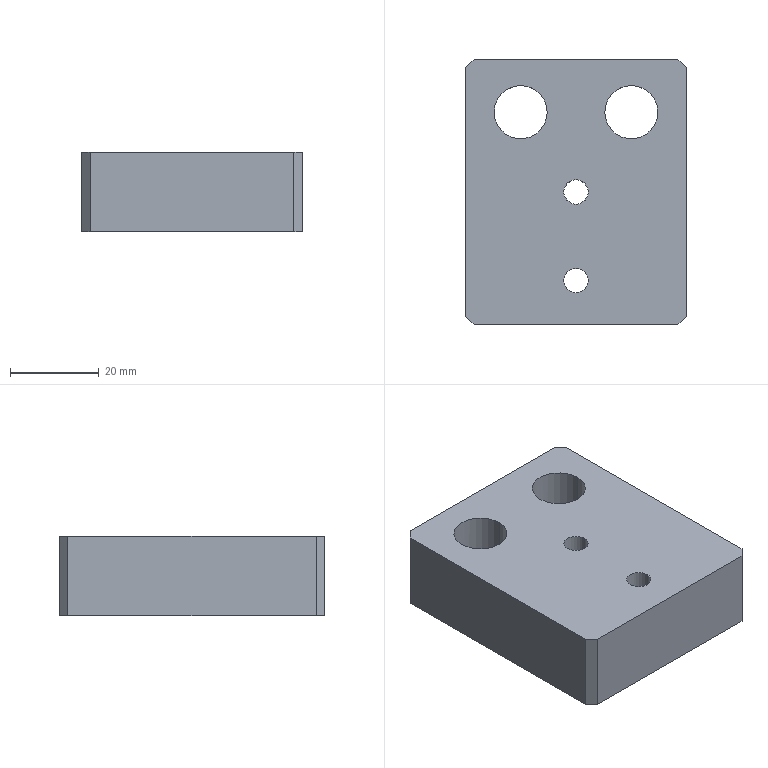Part | SolidWorks | features BaseBody 1 | 1 solid | 28 faces | box 50 x 60 x 18 mm | volume 48136 mm3 | cylinder 16 | plane 12 | commonest cylinder face diameters 4.2 x4 5.5 x4 10 x4 12 x4
STEP:
#1=CARTESIAN_POINT('',(5.,10.,-3.3));
#2=VERTEX_POINT('',#1);
#3=CARTESIAN_POINT('',(-5.,10.,-3.3));
#4=VERTEX_POINT('',#3);
#5=CARTESIAN_POINT('',(0.,10.,-3.3));
#6=DIRECTION('',(0.,0.,-1.));
#7=DIRECTION('',(-1.,0.,0.));
#8=AXIS2_PLACEMENT_3D('',#5,#6,#7);
#9=CIRCLE('',#8,5.);
#10=EDGE_CURVE('',#2,#4,#9,.T.);
#11=ORIENTED_EDGE('',*,*,#10,.F.);
#12=CARTESIAN_POINT('',(5.,10.,-9.));
#13=VERTEX_POINT('',#12);
#14=CARTESIAN_POINT('',(5.,10.,-9.));
#15=DIRECTION('',(0.,0.,-1.));
#16=VECTOR('',#15,1000.);
#17=LINE('',#14,#16);
#18=EDGE_CURVE('',#2,#13,#17,.T.);
#19=ORIENTED_EDGE('',*,*,#18,.T.);
#20=CARTESIAN_POINT('',(-5.,10.,-9.));
#21=VERTEX_POINT('',#20);
#22=CARTESIAN_POINT('',(0.,10.,-9.));
#23=DIRECTION('',(0.,0.,-1.));
#24=DIRECTION('',(-1.,0.,0.));
#25=AXIS2_PLACEMENT_3D('',#22,#23,#24);
#26=CIRCLE('',#25,5.);
#27=EDGE_CURVE('',#13,#21,#26,.T.);
#28=ORIENTED_EDGE('',*,*,#27,.T.);
#29=CARTESIAN_POINT('',(-5.,10.,-9.));
#30=DIRECTION('',(0.,0.,-1.));
#31=VECTOR('',#30,1000.);
#32=LINE('',#29,#31);
#33=EDGE_CURVE('',#4,#21,#32,.T.);
#34=ORIENTED_EDGE('',*,*,#33,.F.);
#35=EDGE_LOOP('',(#11,#19,#28,#34));
#36=FACE_OUTER_BOUND('',#35,.T.);
#37=CARTESIAN_POINT('',(0.,10.,-9.));
#38=DIRECTION('',(0.,0.,-1.));
#39=DIRECTION('',(-1.,0.,0.));
#40=AXIS2_PLACEMENT_3D('',#37,#38,#39);
#41=CYLINDRICAL_SURFACE('',#40,5.);
#42=ADVANCED_FACE('',(#36),#41,.F.);
#43=CARTESIAN_POINT('',(2.75,10.,9.));
#44=VERTEX_POINT('',#43);
#45=CARTESIAN_POINT('',(-2.75,10.,9.));
#46=VERTEX_POINT('',#45);
#47=CARTESIAN_POINT('',(0.,10.,9.));
#48=DIRECTION('',(0.,0.,-1.));
#49=DIRECTION('',(-1.,0.,0.));
#50=AXIS2_PLACEMENT_3D('',#47,#48,#49);
#51=CIRCLE('',#50,2.75);
#52=EDGE_CURVE('',#44,#46,#51,.T.);
#53=ORIENTED_EDGE('',*,*,#52,.F.);
#54=CARTESIAN_POINT('',(2.75,10.,-3.3));
#55=VERTEX_POINT('',#54);
#56=CARTESIAN_POINT('',(2.75,10.,-9.));
#57=DIRECTION('',(0.,0.,-1.));
#58=VECTOR('',#57,1000.);
#59=LINE('',#56,#58);
#60=EDGE_CURVE('',#44,#55,#59,.T.);
#61=ORIENTED_EDGE('',*,*,#60,.T.);
#62=CARTESIAN_POINT('',(-2.75,10.,-3.3));
#63=VERTEX_POINT('',#62);
#64=CARTESIAN_POINT('',(0.,10.,-3.3));
#65=DIRECTION('',(0.,0.,-1.));
#66=DIRECTION('',(-1.,0.,0.));
#67=AXIS2_PLACEMENT_3D('',#64,#65,#66);
#68=CIRCLE('',#67,2.75);
#69=EDGE_CURVE('',#55,#63,#68,.T.);
#70=ORIENTED_EDGE('',*,*,#69,.T.);
#71=CARTESIAN_POINT('',(-2.75,10.,-9.));
#72=DIRECTION('',(0.,0.,-1.));
#73=VECTOR('',#72,1000.);
#74=LINE('',#71,#73);
#75=EDGE_CURVE('',#46,#63,#74,.T.);
#76=ORIENTED_EDGE('',*,*,#75,.F.);
#77=EDGE_LOOP('',(#53,#61,#70,#76));
#78=FACE_OUTER_BOUND('',#77,.T.);
#79=CARTESIAN_POINT('',(0.,10.,-9.));
#80=DIRECTION('',(0.,0.,-1.));
#81=DIRECTION('',(-1.,0.,0.));
#82=AXIS2_PLACEMENT_3D('',#79,#80,#81);
#83=CYLINDRICAL_SURFACE('',#82,2.75);
#84=ADVANCED_FACE('',(#78),#83,.F.);
#85=CARTESIAN_POINT('',(5.,30.,-3.3));
#86=VERTEX_POINT('',#85);
#87=CARTESIAN_POINT('',(-5.,30.,-3.3));
#88=VERTEX_POINT('',#87);
#89=CARTESIAN_POINT('',(0.,30.,-3.3));
#90=DIRECTION('',(0.,0.,-1.));
#91=DIRECTION('',(-1.,0.,0.));
#92=AXIS2_PLACEMENT_3D('',#89,#90,#91);
#93=CIRCLE('',#92,5.);
#94=EDGE_CURVE('',#86,#88,#93,.T.);
#95=ORIENTED_EDGE('',*,*,#94,.F.);
#96=CARTESIAN_POINT('',(5.,30.,-9.));
#97=VERTEX_POINT('',#96);
#98=CARTESIAN_POINT('',(5.,30.,-9.));
#99=DIRECTION('',(0.,0.,-1.));
#100=VECTOR('',#99,1000.);
#101=LINE('',#98,#100);
#102=EDGE_CURVE('',#86,#97,#101,.T.);
#103=ORIENTED_EDGE('',*,*,#102,.T.);
#104=CARTESIAN_POINT('',(-5.,30.,-9.));
#105=VERTEX_POINT('',#104);
#106=CARTESIAN_POINT('',(0.,30.,-9.));
#107=DIRECTION('',(0.,0.,-1.));
#108=DIRECTION('',(-1.,0.,0.));
#109=AXIS2_PLACEMENT_3D('',#106,#107,#108);
#110=CIRCLE('',#109,5.);
#111=EDGE_CURVE('',#97,#105,#110,.T.);
#112=ORIENTED_EDGE('',*,*,#111,.T.);
#113=CARTESIAN_POINT('',(-5.,30.,-9.));
#114=DIRECTION('',(0.,0.,-1.));
#115=VECTOR('',#114,1000.);
#116=LINE('',#113,#115);
#117=EDGE_CURVE('',#88,#105,#116,.T.);
#118=ORIENTED_EDGE('',*,*,#117,.F.);
#119=EDGE_LOOP('',(#95,#103,#112,#118));
#120=FACE_OUTER_BOUND('',#119,.T.);
#121=CARTESIAN_POINT('',(0.,30.,-9.));
#122=DIRECTION('',(0.,0.,-1.));
#123=DIRECTION('',(-1.,0.,0.));
#124=AXIS2_PLACEMENT_3D('',#121,#122,#123);
#125=CYLINDRICAL_SURFACE('',#124,5.);
#126=ADVANCED_FACE('',(#120),#125,.F.);
#127=CARTESIAN_POINT('',(2.75,30.,9.));
#128=VERTEX_POINT('',#127);
#129=CARTESIAN_POINT('',(-2.75,30.,9.));
#130=VERTEX_POINT('',#129);
#131=CARTESIAN_POINT('',(0.,30.,9.));
#132=DIRECTION('',(0.,0.,-1.));
#133=DIRECTION('',(-1.,0.,0.));
#134=AXIS2_PLACEMENT_3D('',#131,#132,#133);
#135=CIRCLE('',#134,2.75);
#136=EDGE_CURVE('',#128,#130,#135,.T.);
#137=ORIENTED_EDGE('',*,*,#136,.F.);
#138=CARTESIAN_POINT('',(2.75,30.,-3.3));
#139=VERTEX_POINT('',#138);
#140=CARTESIAN_POINT('',(2.75,30.,-9.));
#141=DIRECTION('',(0.,0.,-1.));
#142=VECTOR('',#141,1000.);
#143=LINE('',#140,#142);
#144=EDGE_CURVE('',#128,#139,#143,.T.);
#145=ORIENTED_EDGE('',*,*,#144,.T.);
#146=CARTESIAN_POINT('',(-2.75,30.,-3.3));
#147=VERTEX_POINT('',#146);
#148=CARTESIAN_POINT('',(0.,30.,-3.3));
#149=DIRECTION('',(0.,0.,-1.));
#150=DIRECTION('',(-1.,0.,0.));
#151=AXIS2_PLACEMENT_3D('',#148,#149,#150);
#152=CIRCLE('',#151,2.75);
#153=EDGE_CURVE('',#139,#147,#152,.T.);
#154=ORIENTED_EDGE('',*,*,#153,.T.);
#155=CARTESIAN_POINT('',(-2.75,30.,-9.));
#156=DIRECTION('',(0.,0.,-1.));
#157=VECTOR('',#156,1000.);
#158=LINE('',#155,#157);
#159=EDGE_CURVE('',#130,#147,#158,.T.);
#160=ORIENTED_EDGE('',*,*,#159,.F.);
#161=EDGE_LOOP('',(#137,#145,#154,#160));
#162=FACE_OUTER_BOUND('',#161,.T.);
#163=CARTESIAN_POINT('',(0.,30.,-9.));
#164=DIRECTION('',(0.,0.,-1.));
#165=DIRECTION('',(-1.,0.,0.));
#166=AXIS2_PLACEMENT_3D('',#163,#164,#165);
#167=CYLINDRICAL_SURFACE('',#166,2.75);
#168=ADVANCED_FACE('',(#162),#167,.F.);
#169=CARTESIAN_POINT('',(-12.5,54.,-2.1));
#170=VERTEX_POINT('',#169);
#171=CARTESIAN_POINT('',(-12.5,54.,2.1));
#172=VERTEX_POINT('',#171);
#173=CARTESIAN_POINT('',(-12.5,54.,-2.1));
#174=CARTESIAN_POINT('',(-12.64,54.,-2.1));
#175=CARTESIAN_POINT('',(-12.777,53.995,-2.086));
#176=CARTESIAN_POINT('',(-13.047,53.977,-2.032));
#177=CARTESIAN_POINT('',(-13.181,53.963,-1.991));
#178=CARTESIAN_POINT('',(-13.435,53.928,-1.885));
#179=CARTESIAN_POINT('',(-13.555,53.908,-1.821));
#180=CARTESIAN_POINT('',(-13.782,53.862,-1.669));
#181=CARTESIAN_POINT('',(-13.889,53.838,-1.581));
#182=CARTESIAN_POINT('',(-14.177,53.764,-1.293));
#183=CARTESIAN_POINT('',(-14.333,53.714,-1.06));
#184=CARTESIAN_POINT('',(-14.491,53.66,-0.6824));
#185=CARTESIAN_POINT('',(-14.532,53.646,-0.549));
#186=CARTESIAN_POINT('',(-14.586,53.626,-0.2775));
#187=CARTESIAN_POINT('',(-14.6,53.621,-0.1406));
#188=CARTESIAN_POINT('',(-14.6,53.62,0.1358));
#189=CARTESIAN_POINT('',(-14.586,53.626,0.2761));
#190=CARTESIAN_POINT('',(-14.532,53.645,0.5464));
#191=CARTESIAN_POINT('',(-14.492,53.66,0.6778));
#192=CARTESIAN_POINT('',(-14.386,53.696,0.9335));
#193=CARTESIAN_POINT('',(-14.321,53.717,1.054));
#194=CARTESIAN_POINT('',(-14.17,53.763,1.281));
#195=CARTESIAN_POINT('',(-14.082,53.788,1.388));
#196=CARTESIAN_POINT('',(-13.889,53.838,1.581));
#197=CARTESIAN_POINT('',(-13.785,53.862,1.667));
#198=CARTESIAN_POINT('',(-13.558,53.907,1.819));
#199=CARTESIAN_POINT('',(-13.435,53.928,1.885));
#200=CARTESIAN_POINT('',(-13.056,53.98,2.043));
#201=CARTESIAN_POINT('',(-12.78,54.,2.1));
#202=CARTESIAN_POINT('',(-12.5,54.,2.1));
#203=B_SPLINE_CURVE_WITH_KNOTS('',3,(#173,#174,#175,#176,#177,#178,#179,#180,#181,#182,#183,#184,#185,#186,#187,#188,#189,#190,#191,#192,#193,#194,#195,#196,#197,#198,#199,#200,#201,#202),.UNSPECIFIED.,.F.,.F.,(4,2,2,2,2,2,2,2,2,2,2,2,2,2,4),(0.,0.0004135,0.000827,0.00124,0.001654,0.002481,0.002894,0.003308,0.003721,0.004135,0.004548,0.004962,0.005375,0.005789,0.006616),.UNSPECIFIED.);
#204=EDGE_CURVE('',#170,#172,#203,.T.);
#205=ORIENTED_EDGE('',*,*,#204,.F.);
#206=CARTESIAN_POINT('',(-12.5,60.,-2.1));
#207=VERTEX_POINT('',#206);
#208=CARTESIAN_POINT('',(-12.5,60.,-2.1));
#209=DIRECTION('',(0.,1.,0.));
#210=VECTOR('',#209,1000.);
#211=LINE('',#208,#210);
#212=EDGE_CURVE('',#170,#207,#211,.T.);
#213=ORIENTED_EDGE('',*,*,#212,.T.);
#214=CARTESIAN_POINT('',(-12.5,60.,2.1));
#215=VERTEX_POINT('',#214);
#216=CARTESIAN_POINT('',(-12.5,60.,0.));
#217=DIRECTION('',(0.,1.,0.));
#218=DIRECTION('',(0.,0.,1.));
#219=AXIS2_PLACEMENT_3D('',#216,#217,#218);
#220=CIRCLE('',#219,2.1);
#221=EDGE_CURVE('',#207,#215,#220,.T.);
#222=ORIENTED_EDGE('',*,*,#221,.T.);
#223=CARTESIAN_POINT('',(-12.5,60.,2.1));
#224=DIRECTION('',(0.,1.,0.));
#225=VECTOR('',#224,1000.);
#226=LINE('',#223,#225);
#227=EDGE_CURVE('',#172,#215,#226,.T.);
#228=ORIENTED_EDGE('',*,*,#227,.F.);
#229=EDGE_LOOP('',(#205,#213,#222,#228));
#230=FACE_OUTER_BOUND('',#229,.T.);
#231=CARTESIAN_POINT('',(-12.5,60.,0.));
#232=DIRECTION('',(0.,1.,0.));
#233=DIRECTION('',(0.,0.,1.));
#234=AXIS2_PLACEMENT_3D('',#231,#232,#233);
#235=CYLINDRICAL_SURFACE('',#234,2.1);
#236=ADVANCED_FACE('',(#230),#235,.F.);
#237=CARTESIAN_POINT('',(12.5,54.,-2.1));
#238=VERTEX_POINT('',#237);
#239=CARTESIAN_POINT('',(12.5,54.,2.1));
#240=VERTEX_POINT('',#239);
#241=CARTESIAN_POINT('',(12.5,54.,-2.1));
#242=CARTESIAN_POINT('',(12.36,54.,-2.1));
#243=CARTESIAN_POINT('',(12.223,53.995,-2.086));
#244=CARTESIAN_POINT('',(11.953,53.977,-2.032));
#245=CARTESIAN_POINT('',(11.819,53.963,-1.991));
#246=CARTESIAN_POINT('',(11.565,53.928,-1.885));
#247=CARTESIAN_POINT('',(11.445,53.908,-1.821));
#248=CARTESIAN_POINT('',(11.218,53.862,-1.669));
#249=CARTESIAN_POINT('',(11.111,53.838,-1.581));
#250=CARTESIAN_POINT('',(10.823,53.764,-1.293));
#251=CARTESIAN_POINT('',(10.667,53.714,-1.06));
#252=CARTESIAN_POINT('',(10.509,53.66,-0.6824));
#253=CARTESIAN_POINT('',(10.468,53.646,-0.549));
#254=CARTESIAN_POINT('',(10.414,53.626,-0.2775));
#255=CARTESIAN_POINT('',(10.4,53.621,-0.1406));
#256=CARTESIAN_POINT('',(10.4,53.62,0.1358));
#257=CARTESIAN_POINT('',(10.414,53.626,0.2761));
#258=CARTESIAN_POINT('',(10.468,53.645,0.5464));
#259=CARTESIAN_POINT('',(10.508,53.66,0.6778));
#260=CARTESIAN_POINT('',(10.614,53.696,0.9335));
#261=CARTESIAN_POINT('',(10.679,53.717,1.054));
#262=CARTESIAN_POINT('',(10.83,53.763,1.281));
#263=CARTESIAN_POINT('',(10.918,53.788,1.388));
#264=CARTESIAN_POINT('',(11.111,53.838,1.581));
#265=CARTESIAN_POINT('',(11.215,53.862,1.667));
#266=CARTESIAN_POINT('',(11.442,53.907,1.819));
#267=CARTESIAN_POINT('',(11.565,53.928,1.885));
#268=CARTESIAN_POINT('',(11.944,53.98,2.043));
#269=CARTESIAN_POINT('',(12.22,54.,2.1));
#270=CARTESIAN_POINT('',(12.5,54.,2.1));
#271=B_SPLINE_CURVE_WITH_KNOTS('',3,(#241,#242,#243,#244,#245,#246,#247,#248,#249,#250,#251,#252,#253,#254,#255,#256,#257,#258,#259,#260,#261,#262,#263,#264,#265,#266,#267,#268,#269,#270),.UNSPECIFIED.,.F.,.F.,(4,2,2,2,2,2,2,2,2,2,2,2,2,2,4),(0.,0.0004135,0.000827,0.00124,0.001654,0.002481,0.002894,0.003308,0.003721,0.004135,0.004548,0.004962,0.005375,0.005789,0.006616),.UNSPECIFIED.);
#272=EDGE_CURVE('',#238,#240,#271,.T.);
#273=ORIENTED_EDGE('',*,*,#272,.F.);
#274=CARTESIAN_POINT('',(12.5,60.,-2.1));
#275=VERTEX_POINT('',#274);
#276=CARTESIAN_POINT('',(12.5,60.,-2.1));
#277=DIRECTION('',(0.,1.,0.));
#278=VECTOR('',#277,1000.);
#279=LINE('',#276,#278);
#280=EDGE_CURVE('',#238,#275,#279,.T.);
#281=ORIENTED_EDGE('',*,*,#280,.T.);
#282=CARTESIAN_POINT('',(12.5,60.,2.1));
#283=VERTEX_POINT('',#282);
#284=CARTESIAN_POINT('',(12.5,60.,0.));
#285=DIRECTION('',(0.,1.,0.));
#286=DIRECTION('',(0.,0.,1.));
#287=AXIS2_PLACEMENT_3D('',#284,#285,#286);
#288=CIRCLE('',#287,2.1);
#289=EDGE_CURVE('',#275,#283,#288,.T.);
#290=ORIENTED_EDGE('',*,*,#289,.T.);
#291=CARTESIAN_POINT('',(12.5,60.,2.1));
#292=DIRECTION('',(0.,1.,0.));
#293=VECTOR('',#292,1000.);
#294=LINE('',#291,#293);
#295=EDGE_CURVE('',#240,#283,#294,.T.);
#296=ORIENTED_EDGE('',*,*,#295,.F.);
#297=EDGE_LOOP('',(#273,#281,#290,#296));
#298=FACE_OUTER_BOUND('',#297,.T.);
#299=CARTESIAN_POINT('',(12.5,60.,0.));
#300=DIRECTION('',(0.,1.,0.));
#301=DIRECTION('',(0.,0.,1.));
#302=AXIS2_PLACEMENT_3D('',#299,#300,#301);
#303=CYLINDRICAL_SURFACE('',#302,2.1);
#304=ADVANCED_FACE('',(#298),#303,.F.);
#305=CARTESIAN_POINT('',(6.5,48.,-9.));
#306=VERTEX_POINT('',#305);
#307=CARTESIAN_POINT('',(18.5,48.,-9.));
#308=VERTEX_POINT('',#307);
#309=CARTESIAN_POINT('',(12.5,48.,-9.));
#310=DIRECTION('',(0.,0.,1.));
#311=DIRECTION('',(1.,0.,0.));
#312=AXIS2_PLACEMENT_3D('',#309,#310,#311);
#313=CIRCLE('',#312,6.);
#314=EDGE_CURVE('',#306,#308,#313,.T.);
#315=ORIENTED_EDGE('',*,*,#314,.F.);
#316=CARTESIAN_POINT('',(6.5,48.,9.));
#317=VERTEX_POINT('',#316);
#318=CARTESIAN_POINT('',(6.5,48.,-9.));
#319=DIRECTION('',(0.,0.,1.));
#320=VECTOR('',#319,1000.);
#321=LINE('',#318,#320);
#322=EDGE_CURVE('',#306,#317,#321,.T.);
#323=ORIENTED_EDGE('',*,*,#322,.T.);
#324=CARTESIAN_POINT('',(18.5,48.,9.));
#325=VERTEX_POINT('',#324);
#326=CARTESIAN_POINT('',(12.5,48.,9.));
#327=DIRECTION('',(0.,0.,1.));
#328=DIRECTION('',(1.,0.,0.));
#329=AXIS2_PLACEMENT_3D('',#326,#327,#328);
#330=CIRCLE('',#329,6.);
#331=EDGE_CURVE('',#317,#325,#330,.T.);
#332=ORIENTED_EDGE('',*,*,#331,.T.);
#333=CARTESIAN_POINT('',(18.5,48.,-9.));
#334=DIRECTION('',(0.,0.,1.));
#335=VECTOR('',#334,1000.);
#336=LINE('',#333,#335);
#337=EDGE_CURVE('',#308,#325,#336,.T.);
#338=ORIENTED_EDGE('',*,*,#337,.F.);
#339=EDGE_LOOP('',(#315,#323,#332,#338));
#340=FACE_OUTER_BOUND('',#339,.T.);
#341=CARTESIAN_POINT('',(12.5,48.,-9.));
#342=DIRECTION('',(0.,0.,1.));
#343=DIRECTION('',(1.,0.,0.));
#344=AXIS2_PLACEMENT_3D('',#341,#342,#343);
#345=CYLINDRICAL_SURFACE('',#344,6.);
#346=ADVANCED_FACE('',(#340),#345,.F.);
#347=CARTESIAN_POINT('',(-18.5,48.,-9.));
#348=VERTEX_POINT('',#347);
#349=CARTESIAN_POINT('',(-6.5,48.,-9.));
#350=VERTEX_POINT('',#349);
#351=CARTESIAN_POINT('',(-12.5,48.,-9.));
#352=DIRECTION('',(0.,0.,1.));
#353=DIRECTION('',(1.,0.,0.));
#354=AXIS2_PLACEMENT_3D('',#351,#352,#353);
#355=CIRCLE('',#354,6.);
#356=EDGE_CURVE('',#348,#350,#355,.T.);
#357=ORIENTED_EDGE('',*,*,#356,.F.);
#358=CARTESIAN_POINT('',(-18.5,48.,9.));
#359=VERTEX_POINT('',#358);
#360=CARTESIAN_POINT('',(-18.5,48.,-9.));
#361=DIRECTION('',(0.,0.,1.));
#362=VECTOR('',#361,1000.);
#363=LINE('',#360,#362);
#364=EDGE_CURVE('',#348,#359,#363,.T.);
#365=ORIENTED_EDGE('',*,*,#364,.T.);
#366=CARTESIAN_POINT('',(-6.5,48.,9.));
#367=VERTEX_POINT('',#366);
#368=CARTESIAN_POINT('',(-12.5,48.,9.));
#369=DIRECTION('',(0.,0.,1.));
#370=DIRECTION('',(1.,0.,0.));
#371=AXIS2_PLACEMENT_3D('',#368,#369,#370);
#372=CIRCLE('',#371,6.);
#373=EDGE_CURVE('',#359,#367,#372,.T.);
#374=ORIENTED_EDGE('',*,*,#373,.T.);
#375=CARTESIAN_POINT('',(-6.5,48.,-9.));
#376=DIRECTION('',(0.,0.,1.));
#377=VECTOR('',#376,1000.);
#378=LINE('',#375,#377);
#379=EDGE_CURVE('',#350,#367,#378,.T.);
#380=ORIENTED_EDGE('',*,*,#379,.F.);
#381=EDGE_LOOP('',(#357,#365,#374,#380));
#382=FACE_OUTER_BOUND('',#381,.T.);
#383=CARTESIAN_POINT('',(-12.5,48.,-9.));
#384=DIRECTION('',(0.,0.,1.));
#385=DIRECTION('',(1.,0.,0.));
#386=AXIS2_PLACEMENT_3D('',#383,#384,#385);
#387=CYLINDRICAL_SURFACE('',#386,6.);
#388=ADVANCED_FACE('',(#382),#387,.F.);
#389=CARTESIAN_POINT('',(23.,0.,9.));
#390=VERTEX_POINT('',#389);
#391=CARTESIAN_POINT('',(25.,2.,9.));
#392=VERTEX_POINT('',#391);
#393=CARTESIAN_POINT('',(25.,2.,9.));
#394=DIRECTION('',(0.7071,0.7071,0.));
#395=VECTOR('',#394,1000.);
#396=LINE('',#393,#395);
#397=EDGE_CURVE('',#390,#392,#396,.T.);
#398=ORIENTED_EDGE('',*,*,#397,.F.);
#399=CARTESIAN_POINT('',(23.,0.,-9.));
#400=VERTEX_POINT('',#399);
#401=CARTESIAN_POINT('',(23.,0.,0.));
#402=DIRECTION('',(0.,0.,1.));
#403=VECTOR('',#402,1000.);
#404=LINE('',#401,#403);
#405=EDGE_CURVE('',#400,#390,#404,.T.);
#406=ORIENTED_EDGE('',*,*,#405,.F.);
#407=CARTESIAN_POINT('',(25.,2.,-9.));
#408=VERTEX_POINT('',#407);
#409=CARTESIAN_POINT('',(25.,2.,-9.));
#410=DIRECTION('',(-0.7071,-0.7071,0.));
#411=VECTOR('',#410,1000.);
#412=LINE('',#409,#411);
#413=EDGE_CURVE('',#408,#400,#412,.T.);
#414=ORIENTED_EDGE('',*,*,#413,.F.);
#415=CARTESIAN_POINT('',(25.,2.,-9.));
#416=DIRECTION('',(0.,0.,-1.));
#417=VECTOR('',#416,1000.);
#418=LINE('',#415,#417);
#419=EDGE_CURVE('',#392,#408,#418,.T.);
#420=ORIENTED_EDGE('',*,*,#419,.F.);
#421=EDGE_LOOP('',(#398,#406,#414,#420));
#422=FACE_OUTER_BOUND('',#421,.T.);
#423=CARTESIAN_POINT('',(25.,2.,-9.));
#424=DIRECTION('',(-0.7071,0.7071,0.));
#425=DIRECTION('',(0.,0.,1.));
#426=AXIS2_PLACEMENT_3D('',#423,#424,#425);
#427=PLANE('',#426);
#428=ADVANCED_FACE('',(#422),#427,.F.);
#429=CARTESIAN_POINT('',(25.,58.,9.));
#430=VERTEX_POINT('',#429);
#431=CARTESIAN_POINT('',(23.,60.,9.));
#432=VERTEX_POINT('',#431);
#433=CARTESIAN_POINT('',(23.,60.,9.));
#434=DIRECTION('',(-0.7071,0.7071,0.));
#435=VECTOR('',#434,1000.);
#436=LINE('',#433,#435);
#437=EDGE_CURVE('',#430,#432,#436,.T.);
#438=ORIENTED_EDGE('',*,*,#437,.F.);
#439=CARTESIAN_POINT('',(25.,58.,-9.));
#440=VERTEX_POINT('',#439);
#441=CARTESIAN_POINT('',(25.,58.,9.));
#442=DIRECTION('',(0.,0.,1.));
#443=VECTOR('',#442,1000.);
#444=LINE('',#441,#443);
#445=EDGE_CURVE('',#440,#430,#444,.T.);
#446=ORIENTED_EDGE('',*,*,#445,.F.);
#447=CARTESIAN_POINT('',(23.,60.,-9.));
#448=VERTEX_POINT('',#447);
#449=CARTESIAN_POINT('',(23.,60.,-9.));
#450=DIRECTION('',(0.7071,-0.7071,0.));
#451=VECTOR('',#450,1000.);
#452=LINE('',#449,#451);
#453=EDGE_CURVE('',#448,#440,#452,.T.);
#454=ORIENTED_EDGE('',*,*,#453,.F.);
#455=CARTESIAN_POINT('',(23.,60.,-9.));
#456=DIRECTION('',(0.,0.,-1.));
#457=VECTOR('',#456,1000.);
#458=LINE('',#455,#457);
#459=EDGE_CURVE('',#432,#448,#458,.T.);
#460=ORIENTED_EDGE('',*,*,#459,.F.);
#461=EDGE_LOOP('',(#438,#446,#454,#460));
#462=FACE_OUTER_BOUND('',#461,.T.);
#463=CARTESIAN_POINT('',(23.,60.,0.));
#464=DIRECTION('',(0.7071,0.7071,0.));
#465=DIRECTION('',(0.,0.,-1.));
#466=AXIS2_PLACEMENT_3D('',#463,#464,#465);
#467=PLANE('',#466);
#468=ADVANCED_FACE('',(#462),#467,.T.);
#469=CARTESIAN_POINT('',(-25.,58.,-9.));
#470=VERTEX_POINT('',#469);
#471=CARTESIAN_POINT('',(-23.,60.,-9.));
#472=VERTEX_POINT('',#471);
#473=CARTESIAN_POINT('',(-23.,60.,-9.));
#474=DIRECTION('',(0.7071,0.7071,0.));
#475=VECTOR('',#474,1000.);
#476=LINE('',#473,#475);
#477=EDGE_CURVE('',#470,#472,#476,.T.);
#478=ORIENTED_EDGE('',*,*,#477,.F.);
#479=CARTESIAN_POINT('',(-25.,58.,9.));
#480=VERTEX_POINT('',#479);
#481=CARTESIAN_POINT('',(-25.,58.,-9.));
#482=DIRECTION('',(0.,0.,-1.));
#483=VECTOR('',#482,1000.);
#484=LINE('',#481,#483);
#485=EDGE_CURVE('',#480,#470,#484,.T.);
#486=ORIENTED_EDGE('',*,*,#485,.F.);
#487=CARTESIAN_POINT('',(-23.,60.,9.));
#488=VERTEX_POINT('',#487);
#489=CARTESIAN_POINT('',(-23.,60.,9.));
#490=DIRECTION('',(-0.7071,-0.7071,0.));
#491=VECTOR('',#490,1000.);
#492=LINE('',#489,#491);
#493=EDGE_CURVE('',#488,#480,#492,.T.);
#494=ORIENTED_EDGE('',*,*,#493,.F.);
#495=CARTESIAN_POINT('',(-23.,60.,9.));
#496=DIRECTION('',(0.,0.,1.));
#497=VECTOR('',#496,1000.);
#498=LINE('',#495,#497);
#499=EDGE_CURVE('',#472,#488,#498,.T.);
#500=ORIENTED_EDGE('',*,*,#499,.F.);
#501=EDGE_LOOP('',(#478,#486,#494,#500));
#502=FACE_OUTER_BOUND('',#501,.T.);
#503=CARTESIAN_POINT('',(-23.,60.,0.));
#504=DIRECTION('',(-0.7071,0.7071,0.));
#505=DIRECTION('',(0.,0.,1.));
#506=AXIS2_PLACEMENT_3D('',#503,#504,#505);
#507=PLANE('',#506);
#508=ADVANCED_FACE('',(#502),#507,.T.);
#509=CARTESIAN_POINT('',(-23.,0.,-9.));
#510=VERTEX_POINT('',#509);
#511=CARTESIAN_POINT('',(-25.,2.,-9.));
#512=VERTEX_POINT('',#511);
#513=CARTESIAN_POINT('',(-25.,2.,-9.));
#514=DIRECTION('',(-0.7071,0.7071,0.));
#515=VECTOR('',#514,1000.);
#516=LINE('',#513,#515);
#517=EDGE_CURVE('',#510,#512,#516,.T.);
#518=ORIENTED_EDGE('',*,*,#517,.F.);
#519=CARTESIAN_POINT('',(-23.,0.,9.));
#520=VERTEX_POINT('',#519);
#521=CARTESIAN_POINT('',(-23.,0.,0.));
#522=DIRECTION('',(0.,0.,-1.));
#523=VECTOR('',#522,1000.);
#524=LINE('',#521,#523);
#525=EDGE_CURVE('',#520,#510,#524,.T.);
#526=ORIENTED_EDGE('',*,*,#525,.F.);
#527=CARTESIAN_POINT('',(-25.,2.,9.));
#528=VERTEX_POINT('',#527);
#529=CARTESIAN_POINT('',(-25.,2.,9.));
#530=DIRECTION('',(0.7071,-0.7071,0.));
#531=VECTOR('',#530,1000.);
#532=LINE('',#529,#531);
#533=EDGE_CURVE('',#528,#520,#532,.T.);
#534=ORIENTED_EDGE('',*,*,#533,.F.);
#535=CARTESIAN_POINT('',(-25.,2.,-9.));
#536=DIRECTION('',(0.,0.,1.));
#537=VECTOR('',#536,1000.);
#538=LINE('',#535,#537);
#539=EDGE_CURVE('',#512,#528,#538,.T.);
#540=ORIENTED_EDGE('',*,*,#539,.F.);
#541=EDGE_LOOP('',(#518,#526,#534,#540));
#542=FACE_OUTER_BOUND('',#541,.T.);
#543=CARTESIAN_POINT('',(-25.,2.,-9.));
#544=DIRECTION('',(0.7071,0.7071,0.));
#545=DIRECTION('',(0.,0.,-1.));
#546=AXIS2_PLACEMENT_3D('',#543,#544,#545);
#547=PLANE('',#546);
#548=ADVANCED_FACE('',(#542),#547,.F.);
#549=CARTESIAN_POINT('',(0.,10.,-3.3));
#550=DIRECTION('',(0.,0.,-1.));
#551=DIRECTION('',(-1.,0.,0.));
#552=AXIS2_PLACEMENT_3D('',#549,#550,#551);
#553=CIRCLE('',#552,2.75);
#554=EDGE_CURVE('',#63,#55,#553,.T.);
#555=ORIENTED_EDGE('',*,*,#554,.F.);
#556=ORIENTED_EDGE('',*,*,#69,.F.);
#557=EDGE_LOOP('',(#555,#556));
#558=FACE_BOUND('',#557,.T.);
#559=CARTESIAN_POINT('',(0.,10.,-3.3));
#560=DIRECTION('',(0.,0.,-1.));
#561=DIRECTION('',(-1.,0.,0.));
#562=AXIS2_PLACEMENT_3D('',#559,#560,#561);
#563=CIRCLE('',#562,5.);
#564=EDGE_CURVE('',#4,#2,#563,.T.);
#565=ORIENTED_EDGE('',*,*,#564,.T.);
#566=ORIENTED_EDGE('',*,*,#10,.T.);
#567=EDGE_LOOP('',(#565,#566));
#568=FACE_OUTER_BOUND('',#567,.T.);
#569=CARTESIAN_POINT('',(2.75,10.,-3.3));
#570=DIRECTION('',(0.,0.,1.));
#571=DIRECTION('',(1.,0.,0.));
#572=AXIS2_PLACEMENT_3D('',#569,#570,#571);
#573=PLANE('',#572);
#574=ADVANCED_FACE('',(#558,#568),#573,.F.);
#575=CARTESIAN_POINT('',(0.,30.,-3.3));
#576=DIRECTION('',(0.,0.,-1.));
#577=DIRECTION('',(-1.,0.,0.));
#578=AXIS2_PLACEMENT_3D('',#575,#576,#577);
#579=CIRCLE('',#578,2.75);
#580=EDGE_CURVE('',#147,#139,#579,.T.);
#581=ORIENTED_EDGE('',*,*,#580,.F.);
#582=ORIENTED_EDGE('',*,*,#153,.F.);
#583=EDGE_LOOP('',(#581,#582));
#584=FACE_BOUND('',#583,.T.);
#585=CARTESIAN_POINT('',(0.,30.,-3.3));
#586=DIRECTION('',(0.,0.,-1.));
#587=DIRECTION('',(-1.,0.,0.));
#588=AXIS2_PLACEMENT_3D('',#585,#586,#587);
#589=CIRCLE('',#588,5.);
#590=EDGE_CURVE('',#88,#86,#589,.T.);
#591=ORIENTED_EDGE('',*,*,#590,.T.);
#592=ORIENTED_EDGE('',*,*,#94,.T.);
#593=EDGE_LOOP('',(#591,#592));
#594=FACE_OUTER_BOUND('',#593,.T.);
#595=CARTESIAN_POINT('',(2.75,30.,-3.3));
#596=DIRECTION('',(0.,0.,1.));
#597=DIRECTION('',(1.,0.,0.));
#598=AXIS2_PLACEMENT_3D('',#595,#596,#597);
#599=PLANE('',#598);
#600=ADVANCED_FACE('',(#584,#594),#599,.F.);
#601=CARTESIAN_POINT('',(-25.,0.,9.));
#602=DIRECTION('',(1.,0.,0.));
#603=VECTOR('',#602,1000.);
#604=LINE('',#601,#603);
#605=EDGE_CURVE('',#520,#390,#604,.T.);
#606=ORIENTED_EDGE('',*,*,#605,.F.);
#607=ORIENTED_EDGE('',*,*,#525,.T.);
#608=CARTESIAN_POINT('',(-25.,0.,-9.));
#609=DIRECTION('',(-1.,0.,0.));
#610=VECTOR('',#609,1000.);
#611=LINE('',#608,#610);
#612=EDGE_CURVE('',#400,#510,#611,.T.);
#613=ORIENTED_EDGE('',*,*,#612,.F.);
#614=ORIENTED_EDGE('',*,*,#405,.T.);
#615=EDGE_LOOP('',(#606,#607,#613,#614));
#616=FACE_OUTER_BOUND('',#615,.T.);
#617=CARTESIAN_POINT('',(0.,0.,0.));
#618=DIRECTION('',(0.,1.,0.));
#619=DIRECTION('',(1.,0.,0.));
#620=AXIS2_PLACEMENT_3D('',#617,#618,#619);
#621=PLANE('',#620);
#622=ADVANCED_FACE('',(#616),#621,.F.);
#623=CARTESIAN_POINT('',(12.5,60.,0.));
#624=DIRECTION('',(0.,1.,0.));
#625=DIRECTION('',(0.,0.,1.));
#626=AXIS2_PLACEMENT_3D('',#623,#624,#625);
#627=CIRCLE('',#626,2.1);
#628=EDGE_CURVE('',#283,#275,#627,.T.);
#629=ORIENTED_EDGE('',*,*,#628,.F.);
#630=ORIENTED_EDGE('',*,*,#289,.F.);
#631=EDGE_LOOP('',(#629,#630));
#632=FACE_BOUND('',#631,.T.);
#633=CARTESIAN_POINT('',(-12.5,60.,0.));
#634=DIRECTION('',(0.,1.,0.));
#635=DIRECTION('',(0.,0.,1.));
#636=AXIS2_PLACEMENT_3D('',#633,#634,#635);
#637=CIRCLE('',#636,2.1);
#638=EDGE_CURVE('',#215,#207,#637,.T.);
#639=ORIENTED_EDGE('',*,*,#638,.F.);
#640=ORIENTED_EDGE('',*,*,#221,.F.);
#641=EDGE_LOOP('',(#639,#640));
#642=FACE_BOUND('',#641,.T.);
#643=CARTESIAN_POINT('',(-25.,60.,-9.));
#644=DIRECTION('',(-1.,0.,0.));
#645=VECTOR('',#644,1000.);
#646=LINE('',#643,#645);
#647=EDGE_CURVE('',#448,#472,#646,.T.);
#648=ORIENTED_EDGE('',*,*,#647,.T.);
#649=ORIENTED_EDGE('',*,*,#499,.T.);
#650=CARTESIAN_POINT('',(-25.,60.,9.));
#651=DIRECTION('',(1.,0.,0.));
#652=VECTOR('',#651,1000.);
#653=LINE('',#650,#652);
#654=EDGE_CURVE('',#488,#432,#653,.T.);
#655=ORIENTED_EDGE('',*,*,#654,.T.);
#656=ORIENTED_EDGE('',*,*,#459,.T.);
#657=EDGE_LOOP('',(#648,#649,#655,#656));
#658=FACE_OUTER_BOUND('',#657,.T.);
#659=CARTESIAN_POINT('',(0.,60.,0.));
#660=DIRECTION('',(0.,1.,0.));
#661=DIRECTION('',(1.,0.,0.));
#662=AXIS2_PLACEMENT_3D('',#659,#660,#661);
#663=PLANE('',#662);
#664=ADVANCED_FACE('',(#632,#642,#658),#663,.T.);
#665=CARTESIAN_POINT('',(-12.5,48.,9.));
#666=DIRECTION('',(0.,0.,1.));
#667=DIRECTION('',(1.,0.,0.));
#668=AXIS2_PLACEMENT_3D('',#665,#666,#667);
#669=CIRCLE('',#668,6.);
#670=EDGE_CURVE('',#367,#359,#669,.T.);
#671=ORIENTED_EDGE('',*,*,#670,.F.);
#672=ORIENTED_EDGE('',*,*,#373,.F.);
#673=EDGE_LOOP('',(#671,#672));
#674=FACE_BOUND('',#673,.T.);
#675=CARTESIAN_POINT('',(12.5,48.,9.));
#676=DIRECTION('',(0.,0.,1.));
#677=DIRECTION('',(1.,0.,0.));
#678=AXIS2_PLACEMENT_3D('',#675,#676,#677);
#679=CIRCLE('',#678,6.);
#680=EDGE_CURVE('',#325,#317,#679,.T.);
#681=ORIENTED_EDGE('',*,*,#680,.F.);
#682=ORIENTED_EDGE('',*,*,#331,.F.);
#683=EDGE_LOOP('',(#681,#682));
#684=FACE_BOUND('',#683,.T.);
#685=CARTESIAN_POINT('',(0.,30.,9.));
#686=DIRECTION('',(0.,0.,-1.));
#687=DIRECTION('',(-1.,0.,0.));
#688=AXIS2_PLACEMENT_3D('',#685,#686,#687);
#689=CIRCLE('',#688,2.75);
#690=EDGE_CURVE('',#130,#128,#689,.T.);
#691=ORIENTED_EDGE('',*,*,#690,.T.);
#692=ORIENTED_EDGE('',*,*,#136,.T.);
#693=EDGE_LOOP('',(#691,#692));
#694=FACE_BOUND('',#693,.T.);
#695=CARTESIAN_POINT('',(0.,10.,9.));
#696=DIRECTION('',(0.,0.,-1.));
#697=DIRECTION('',(-1.,0.,0.));
#698=AXIS2_PLACEMENT_3D('',#695,#696,#697);
#699=CIRCLE('',#698,2.75);
#700=EDGE_CURVE('',#46,#44,#699,.T.);
#701=ORIENTED_EDGE('',*,*,#700,.T.);
#702=ORIENTED_EDGE('',*,*,#52,.T.);
#703=EDGE_LOOP('',(#701,#702));
#704=FACE_BOUND('',#703,.T.);
#705=CARTESIAN_POINT('',(-25.,60.,9.));
#706=DIRECTION('',(0.,-1.,0.));
#707=VECTOR('',#706,1000.);
#708=LINE('',#705,#707);
#709=EDGE_CURVE('',#480,#528,#708,.T.);
#710=ORIENTED_EDGE('',*,*,#709,.T.);
#711=ORIENTED_EDGE('',*,*,#533,.T.);
#712=ORIENTED_EDGE('',*,*,#605,.T.);
#713=ORIENTED_EDGE('',*,*,#397,.T.);
#714=CARTESIAN_POINT('',(25.,60.,9.));
#715=DIRECTION('',(0.,-1.,0.));
#716=VECTOR('',#715,1000.);
#717=LINE('',#714,#716);
#718=EDGE_CURVE('',#430,#392,#717,.T.);
#719=ORIENTED_EDGE('',*,*,#718,.F.);
#720=ORIENTED_EDGE('',*,*,#437,.T.);
#721=ORIENTED_EDGE('',*,*,#654,.F.);
#722=ORIENTED_EDGE('',*,*,#493,.T.);
#723=EDGE_LOOP('',(#710,#711,#712,#713,#719,#720,#721,#722));
#724=FACE_OUTER_BOUND('',#723,.T.);
#725=CARTESIAN_POINT('',(-25.,60.,9.));
#726=DIRECTION('',(0.,0.,-1.));
#727=DIRECTION('',(0.,-1.,0.));
#728=AXIS2_PLACEMENT_3D('',#725,#726,#727);
#729=PLANE('',#728);
#730=ADVANCED_FACE('',(#674,#684,#694,#704,#724),#729,.F.);
#731=CARTESIAN_POINT('',(-25.,60.,-9.));
#732=DIRECTION('',(0.,-1.,0.));
#733=VECTOR('',#732,1000.);
#734=LINE('',#731,#733);
#735=EDGE_CURVE('',#470,#512,#734,.T.);
#736=ORIENTED_EDGE('',*,*,#735,.T.);
#737=ORIENTED_EDGE('',*,*,#539,.T.);
#738=ORIENTED_EDGE('',*,*,#709,.F.);
#739=ORIENTED_EDGE('',*,*,#485,.T.);
#740=EDGE_LOOP('',(#736,#737,#738,#739));
#741=FACE_OUTER_BOUND('',#740,.T.);
#742=CARTESIAN_POINT('',(-25.,60.,-9.));
#743=DIRECTION('',(1.,0.,0.));
#744=DIRECTION('',(0.,0.,-1.));
#745=AXIS2_PLACEMENT_3D('',#742,#743,#744);
#746=PLANE('',#745);
#747=ADVANCED_FACE('',(#741),#746,.F.);
#748=CARTESIAN_POINT('',(25.,60.,-9.));
#749=DIRECTION('',(0.,-1.,0.));
#750=VECTOR('',#749,1000.);
#751=LINE('',#748,#750);
#752=EDGE_CURVE('',#440,#408,#751,.T.);
#753=ORIENTED_EDGE('',*,*,#752,.F.);
#754=ORIENTED_EDGE('',*,*,#445,.T.);
#755=ORIENTED_EDGE('',*,*,#718,.T.);
#756=ORIENTED_EDGE('',*,*,#419,.T.);
#757=EDGE_LOOP('',(#753,#754,#755,#756));
#758=FACE_OUTER_BOUND('',#757,.T.);
#759=CARTESIAN_POINT('',(25.,60.,-9.));
#760=DIRECTION('',(-1.,0.,0.));
#761=DIRECTION('',(0.,1.,0.));
#762=AXIS2_PLACEMENT_3D('',#759,#760,#761);
#763=PLANE('',#762);
#764=ADVANCED_FACE('',(#758),#763,.F.);
#765=CARTESIAN_POINT('',(0.,10.,-9.));
#766=DIRECTION('',(0.,0.,-1.));
#767=DIRECTION('',(-1.,0.,0.));
#768=AXIS2_PLACEMENT_3D('',#765,#766,#767);
#769=CIRCLE('',#768,5.);
#770=EDGE_CURVE('',#21,#13,#769,.T.);
#771=ORIENTED_EDGE('',*,*,#770,.F.);
#772=ORIENTED_EDGE('',*,*,#27,.F.);
#773=EDGE_LOOP('',(#771,#772));
#774=FACE_BOUND('',#773,.T.);
#775=CARTESIAN_POINT('',(-12.5,48.,-9.));
#776=DIRECTION('',(0.,0.,1.));
#777=DIRECTION('',(1.,0.,0.));
#778=AXIS2_PLACEMENT_3D('',#775,#776,#777);
#779=CIRCLE('',#778,6.);
#780=EDGE_CURVE('',#350,#348,#779,.T.);
#781=ORIENTED_EDGE('',*,*,#780,.T.);
#782=ORIENTED_EDGE('',*,*,#356,.T.);
#783=EDGE_LOOP('',(#781,#782));
#784=FACE_BOUND('',#783,.T.);
#785=CARTESIAN_POINT('',(12.5,48.,-9.));
#786=DIRECTION('',(0.,0.,1.));
#787=DIRECTION('',(1.,0.,0.));
#788=AXIS2_PLACEMENT_3D('',#785,#786,#787);
#789=CIRCLE('',#788,6.);
#790=EDGE_CURVE('',#308,#306,#789,.T.);
#791=ORIENTED_EDGE('',*,*,#790,.T.);
#792=ORIENTED_EDGE('',*,*,#314,.T.);
#793=EDGE_LOOP('',(#791,#792));
#794=FACE_BOUND('',#793,.T.);
#795=CARTESIAN_POINT('',(0.,30.,-9.));
#796=DIRECTION('',(0.,0.,-1.));
#797=DIRECTION('',(-1.,0.,0.));
#798=AXIS2_PLACEMENT_3D('',#795,#796,#797);
#799=CIRCLE('',#798,5.);
#800=EDGE_CURVE('',#105,#97,#799,.T.);
#801=ORIENTED_EDGE('',*,*,#800,.F.);
#802=ORIENTED_EDGE('',*,*,#111,.F.);
#803=EDGE_LOOP('',(#801,#802));
#804=FACE_BOUND('',#803,.T.);
#805=ORIENTED_EDGE('',*,*,#612,.T.);
#806=ORIENTED_EDGE('',*,*,#517,.T.);
#807=ORIENTED_EDGE('',*,*,#735,.F.);
#808=ORIENTED_EDGE('',*,*,#477,.T.);
#809=ORIENTED_EDGE('',*,*,#647,.F.);
#810=ORIENTED_EDGE('',*,*,#453,.T.);
#811=ORIENTED_EDGE('',*,*,#752,.T.);
#812=ORIENTED_EDGE('',*,*,#413,.T.);
#813=EDGE_LOOP('',(#805,#806,#807,#808,#809,#810,#811,#812));
#814=FACE_OUTER_BOUND('',#813,.T.);
#815=CARTESIAN_POINT('',(-25.,60.,-9.));
#816=DIRECTION('',(0.,0.,1.));
#817=DIRECTION('',(1.,0.,0.));
#818=AXIS2_PLACEMENT_3D('',#815,#816,#817);
#819=PLANE('',#818);
#820=ADVANCED_FACE('',(#774,#784,#794,#804,#814),#819,.F.);
#821=ORIENTED_EDGE('',*,*,#364,.F.);
#822=ORIENTED_EDGE('',*,*,#780,.F.);
#823=ORIENTED_EDGE('',*,*,#379,.T.);
#824=ORIENTED_EDGE('',*,*,#670,.T.);
#825=EDGE_LOOP('',(#821,#822,#823,#824));
#826=FACE_OUTER_BOUND('',#825,.T.);
#827=CARTESIAN_POINT('',(-12.5,54.,2.1));
#828=CARTESIAN_POINT('',(-12.36,54.,2.1));
#829=CARTESIAN_POINT('',(-12.223,53.995,2.086));
#830=CARTESIAN_POINT('',(-11.953,53.977,2.032));
#831=CARTESIAN_POINT('',(-11.819,53.963,1.991));
#832=CARTESIAN_POINT('',(-11.565,53.928,1.885));
#833=CARTESIAN_POINT('',(-11.445,53.908,1.821));
#834=CARTESIAN_POINT('',(-11.218,53.862,1.669));
#835=CARTESIAN_POINT('',(-11.111,53.838,1.581));
#836=CARTESIAN_POINT('',(-10.823,53.764,1.293));
#837=CARTESIAN_POINT('',(-10.667,53.714,1.06));
#838=CARTESIAN_POINT('',(-10.509,53.66,0.6824));
#839=CARTESIAN_POINT('',(-10.468,53.646,0.549));
#840=CARTESIAN_POINT('',(-10.414,53.626,0.2775));
#841=CARTESIAN_POINT('',(-10.4,53.621,0.1406));
#842=CARTESIAN_POINT('',(-10.4,53.62,-0.1358));
#843=CARTESIAN_POINT('',(-10.414,53.626,-0.2761));
#844=CARTESIAN_POINT('',(-10.468,53.645,-0.5464));
#845=CARTESIAN_POINT('',(-10.508,53.66,-0.6778));
#846=CARTESIAN_POINT('',(-10.614,53.696,-0.9335));
#847=CARTESIAN_POINT('',(-10.679,53.717,-1.054));
#848=CARTESIAN_POINT('',(-10.83,53.763,-1.281));
#849=CARTESIAN_POINT('',(-10.918,53.788,-1.388));
#850=CARTESIAN_POINT('',(-11.111,53.838,-1.581));
#851=CARTESIAN_POINT('',(-11.215,53.862,-1.667));
#852=CARTESIAN_POINT('',(-11.442,53.907,-1.819));
#853=CARTESIAN_POINT('',(-11.565,53.928,-1.885));
#854=CARTESIAN_POINT('',(-11.944,53.98,-2.043));
#855=CARTESIAN_POINT('',(-12.22,54.,-2.1));
#856=CARTESIAN_POINT('',(-12.5,54.,-2.1));
#857=B_SPLINE_CURVE_WITH_KNOTS('',3,(#827,#828,#829,#830,#831,#832,#833,#834,#835,#836,#837,#838,#839,#840,#841,#842,#843,#844,#845,#846,#847,#848,#849,#850,#851,#852,#853,#854,#855,#856),.UNSPECIFIED.,.F.,.F.,(4,2,2,2,2,2,2,2,2,2,2,2,2,2,4),(0.006616,0.007029,0.007443,0.007856,0.008269,0.009096,0.00951,0.009923,0.01034,0.01075,0.01116,0.01158,0.01199,0.0124,0.01323),.UNSPECIFIED.);
#858=EDGE_CURVE('',#172,#170,#857,.T.);
#859=ORIENTED_EDGE('',*,*,#858,.T.);
#860=ORIENTED_EDGE('',*,*,#204,.T.);
#861=EDGE_LOOP('',(#859,#860));
#862=FACE_BOUND('',#861,.T.);
#863=CARTESIAN_POINT('',(-12.5,48.,-9.));
#864=DIRECTION('',(0.,0.,1.));
#865=DIRECTION('',(1.,0.,0.));
#866=AXIS2_PLACEMENT_3D('',#863,#864,#865);
#867=CYLINDRICAL_SURFACE('',#866,6.);
#868=ADVANCED_FACE('',(#826,#862),#867,.F.);
#869=ORIENTED_EDGE('',*,*,#322,.F.);
#870=ORIENTED_EDGE('',*,*,#790,.F.);
#871=ORIENTED_EDGE('',*,*,#337,.T.);
#872=ORIENTED_EDGE('',*,*,#680,.T.);
#873=EDGE_LOOP('',(#869,#870,#871,#872));
#874=FACE_OUTER_BOUND('',#873,.T.);
#875=CARTESIAN_POINT('',(12.5,54.,2.1));
#876=CARTESIAN_POINT('',(12.64,54.,2.1));
#877=CARTESIAN_POINT('',(12.777,53.995,2.086));
#878=CARTESIAN_POINT('',(13.047,53.977,2.032));
#879=CARTESIAN_POINT('',(13.181,53.963,1.991));
#880=CARTESIAN_POINT('',(13.435,53.928,1.885));
#881=CARTESIAN_POINT('',(13.555,53.908,1.821));
#882=CARTESIAN_POINT('',(13.782,53.862,1.669));
#883=CARTESIAN_POINT('',(13.889,53.838,1.581));
#884=CARTESIAN_POINT('',(14.177,53.764,1.293));
#885=CARTESIAN_POINT('',(14.333,53.714,1.06));
#886=CARTESIAN_POINT('',(14.491,53.66,0.6824));
#887=CARTESIAN_POINT('',(14.532,53.646,0.549));
#888=CARTESIAN_POINT('',(14.586,53.626,0.2775));
#889=CARTESIAN_POINT('',(14.6,53.621,0.1406));
#890=CARTESIAN_POINT('',(14.6,53.62,-0.1358));
#891=CARTESIAN_POINT('',(14.586,53.626,-0.2761));
#892=CARTESIAN_POINT('',(14.532,53.645,-0.5464));
#893=CARTESIAN_POINT('',(14.492,53.66,-0.6778));
#894=CARTESIAN_POINT('',(14.386,53.696,-0.9335));
#895=CARTESIAN_POINT('',(14.321,53.717,-1.054));
#896=CARTESIAN_POINT('',(14.17,53.763,-1.281));
#897=CARTESIAN_POINT('',(14.082,53.788,-1.388));
#898=CARTESIAN_POINT('',(13.889,53.838,-1.581));
#899=CARTESIAN_POINT('',(13.785,53.862,-1.667));
#900=CARTESIAN_POINT('',(13.558,53.907,-1.819));
#901=CARTESIAN_POINT('',(13.435,53.928,-1.885));
#902=CARTESIAN_POINT('',(13.056,53.98,-2.043));
#903=CARTESIAN_POINT('',(12.78,54.,-2.1));
#904=CARTESIAN_POINT('',(12.5,54.,-2.1));
#905=B_SPLINE_CURVE_WITH_KNOTS('',3,(#875,#876,#877,#878,#879,#880,#881,#882,#883,#884,#885,#886,#887,#888,#889,#890,#891,#892,#893,#894,#895,#896,#897,#898,#899,#900,#901,#902,#903,#904),.UNSPECIFIED.,.F.,.F.,(4,2,2,2,2,2,2,2,2,2,2,2,2,2,4),(0.006616,0.007029,0.007443,0.007856,0.008269,0.009096,0.00951,0.009923,0.01034,0.01075,0.01116,0.01158,0.01199,0.0124,0.01323),.UNSPECIFIED.);
#906=EDGE_CURVE('',#240,#238,#905,.T.);
#907=ORIENTED_EDGE('',*,*,#906,.T.);
#908=ORIENTED_EDGE('',*,*,#272,.T.);
#909=EDGE_LOOP('',(#907,#908));
#910=FACE_BOUND('',#909,.T.);
#911=CARTESIAN_POINT('',(12.5,48.,-9.));
#912=DIRECTION('',(0.,0.,1.));
#913=DIRECTION('',(1.,0.,0.));
#914=AXIS2_PLACEMENT_3D('',#911,#912,#913);
#915=CYLINDRICAL_SURFACE('',#914,6.);
#916=ADVANCED_FACE('',(#874,#910),#915,.F.);
#917=ORIENTED_EDGE('',*,*,#280,.F.);
#918=ORIENTED_EDGE('',*,*,#906,.F.);
#919=ORIENTED_EDGE('',*,*,#295,.T.);
#920=ORIENTED_EDGE('',*,*,#628,.T.);
#921=EDGE_LOOP('',(#917,#918,#919,#920));
#922=FACE_OUTER_BOUND('',#921,.T.);
#923=CARTESIAN_POINT('',(12.5,60.,0.));
#924=DIRECTION('',(0.,1.,0.));
#925=DIRECTION('',(0.,0.,1.));
#926=AXIS2_PLACEMENT_3D('',#923,#924,#925);
#927=CYLINDRICAL_SURFACE('',#926,2.1);
#928=ADVANCED_FACE('',(#922),#927,.F.);
#929=ORIENTED_EDGE('',*,*,#212,.F.);
#930=ORIENTED_EDGE('',*,*,#858,.F.);
#931=ORIENTED_EDGE('',*,*,#227,.T.);
#932=ORIENTED_EDGE('',*,*,#638,.T.);
#933=EDGE_LOOP('',(#929,#930,#931,#932));
#934=FACE_OUTER_BOUND('',#933,.T.);
#935=CARTESIAN_POINT('',(-12.5,60.,0.));
#936=DIRECTION('',(0.,1.,0.));
#937=DIRECTION('',(0.,0.,1.));
#938=AXIS2_PLACEMENT_3D('',#935,#936,#937);
#939=CYLINDRICAL_SURFACE('',#938,2.1);
#940=ADVANCED_FACE('',(#934),#939,.F.);
#941=ORIENTED_EDGE('',*,*,#144,.F.);
#942=ORIENTED_EDGE('',*,*,#690,.F.);
#943=ORIENTED_EDGE('',*,*,#159,.T.);
#944=ORIENTED_EDGE('',*,*,#580,.T.);
#945=EDGE_LOOP('',(#941,#942,#943,#944));
#946=FACE_OUTER_BOUND('',#945,.T.);
#947=CARTESIAN_POINT('',(0.,30.,-9.));
#948=DIRECTION('',(0.,0.,-1.));
#949=DIRECTION('',(-1.,0.,0.));
#950=AXIS2_PLACEMENT_3D('',#947,#948,#949);
#951=CYLINDRICAL_SURFACE('',#950,2.75);
#952=ADVANCED_FACE('',(#946),#951,.F.);
#953=ORIENTED_EDGE('',*,*,#102,.F.);
#954=ORIENTED_EDGE('',*,*,#590,.F.);
#955=ORIENTED_EDGE('',*,*,#117,.T.);
#956=ORIENTED_EDGE('',*,*,#800,.T.);
#957=EDGE_LOOP('',(#953,#954,#955,#956));
#958=FACE_OUTER_BOUND('',#957,.T.);
#959=CARTESIAN_POINT('',(0.,30.,-9.));
#960=DIRECTION('',(0.,0.,-1.));
#961=DIRECTION('',(-1.,0.,0.));
#962=AXIS2_PLACEMENT_3D('',#959,#960,#961);
#963=CYLINDRICAL_SURFACE('',#962,5.);
#964=ADVANCED_FACE('',(#958),#963,.F.);
#965=ORIENTED_EDGE('',*,*,#60,.F.);
#966=ORIENTED_EDGE('',*,*,#700,.F.);
#967=ORIENTED_EDGE('',*,*,#75,.T.);
#968=ORIENTED_EDGE('',*,*,#554,.T.);
#969=EDGE_LOOP('',(#965,#966,#967,#968));
#970=FACE_OUTER_BOUND('',#969,.T.);
#971=CARTESIAN_POINT('',(0.,10.,-9.));
#972=DIRECTION('',(0.,0.,-1.));
#973=DIRECTION('',(-1.,0.,0.));
#974=AXIS2_PLACEMENT_3D('',#971,#972,#973);
#975=CYLINDRICAL_SURFACE('',#974,2.75);
#976=ADVANCED_FACE('',(#970),#975,.F.);
#977=ORIENTED_EDGE('',*,*,#18,.F.);
#978=ORIENTED_EDGE('',*,*,#564,.F.);
#979=ORIENTED_EDGE('',*,*,#33,.T.);
#980=ORIENTED_EDGE('',*,*,#770,.T.);
#981=EDGE_LOOP('',(#977,#978,#979,#980));
#982=FACE_OUTER_BOUND('',#981,.T.);
#983=CARTESIAN_POINT('',(0.,10.,-9.));
#984=DIRECTION('',(0.,0.,-1.));
#985=DIRECTION('',(-1.,0.,0.));
#986=AXIS2_PLACEMENT_3D('',#983,#984,#985);
#987=CYLINDRICAL_SURFACE('',#986,5.);
#988=ADVANCED_FACE('',(#982),#987,.F.);
#989=CLOSED_SHELL('',(#42,#84,#126,#168,#236,#304,#346,#388,#428,#468,#508,#548,#574,#600,#622,#664,#730,#747,#764,#820,#868,#916,#928,#940,#952,#964,#976,#988));
#990=MANIFOLD_SOLID_BREP('',#989);
#991=CARTESIAN_POINT('',(0.,0.,0.));
#992=DIRECTION('',(0.,0.,1.));
#993=DIRECTION('',(1.,0.,0.));
#994=AXIS2_PLACEMENT_3D('',#991,#992,#993);
#995=(LENGTH_UNIT()NAMED_UNIT(*)SI_UNIT(.MILLI.,.METRE.));
#996=UNCERTAINTY_MEASURE_WITH_UNIT(LENGTH_MEASURE(0.00001),#995,'','');
#997=(NAMED_UNIT(*)PLANE_ANGLE_UNIT()SI_UNIT($,.RADIAN.));
#998=(NAMED_UNIT(*)SI_UNIT($,.STERADIAN.)SOLID_ANGLE_UNIT());
#999=(GEOMETRIC_REPRESENTATION_CONTEXT(3)GLOBAL_UNCERTAINTY_ASSIGNED_CONTEXT((#996))GLOBAL_UNIT_ASSIGNED_CONTEXT((#995,#997,#998))REPRESENTATION_CONTEXT('',''));
#1000=ADVANCED_BREP_SHAPE_REPRESENTATION('',(#990,#994),#999);